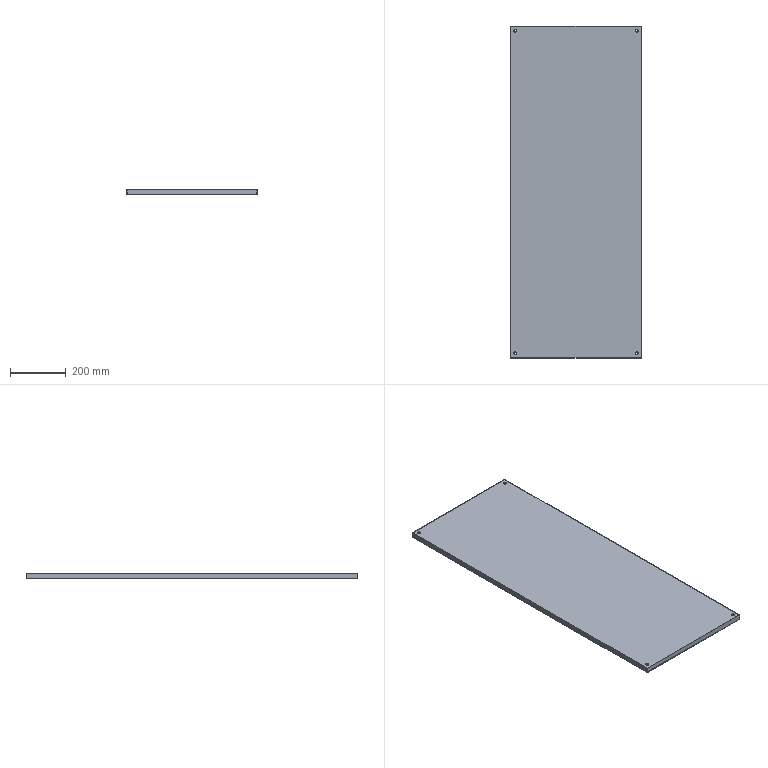Part | SolidWorks | features Extrusion 1, HoleWzd 1, ICE 1, Shell 1 | 1 solid | 32 faces | box 471 x 1196 x 20 mm | volume 1361647 mm3 | cylinder 16 | plane 16 | commonest cylinder face diameters 6.6 x8 11 x8
STEP:
#1=CARTESIAN_POINT('',(-213.,580.75,18.));
#2=VERTEX_POINT('',#1);
#3=CARTESIAN_POINT('',(-224.,580.75,18.));
#4=VERTEX_POINT('',#3);
#5=CARTESIAN_POINT('',(-218.5,580.75,18.));
#6=DIRECTION('',(0.,0.,-1.));
#7=DIRECTION('',(-1.,0.,0.));
#8=AXIS2_PLACEMENT_3D('',#5,#6,#7);
#9=CIRCLE('',#8,5.5);
#10=EDGE_CURVE('',#2,#4,#9,.T.);
#11=ORIENTED_EDGE('',*,*,#10,.T.);
#12=CARTESIAN_POINT('',(-224.,580.75,20.));
#13=VERTEX_POINT('',#12);
#14=CARTESIAN_POINT('',(-224.,580.75,20.));
#15=DIRECTION('',(0.,0.,1.));
#16=VECTOR('',#15,1000.);
#17=LINE('',#14,#16);
#18=EDGE_CURVE('',#4,#13,#17,.T.);
#19=ORIENTED_EDGE('',*,*,#18,.T.);
#20=CARTESIAN_POINT('',(-213.,580.75,20.));
#21=VERTEX_POINT('',#20);
#22=CARTESIAN_POINT('',(-218.5,580.75,20.));
#23=DIRECTION('',(0.,0.,1.));
#24=DIRECTION('',(1.,0.,0.));
#25=AXIS2_PLACEMENT_3D('',#22,#23,#24);
#26=CIRCLE('',#25,5.5);
#27=EDGE_CURVE('',#13,#21,#26,.T.);
#28=ORIENTED_EDGE('',*,*,#27,.T.);
#29=CARTESIAN_POINT('',(-213.,580.75,20.));
#30=DIRECTION('',(0.,0.,1.));
#31=VECTOR('',#30,1000.);
#32=LINE('',#29,#31);
#33=EDGE_CURVE('',#2,#21,#32,.T.);
#34=ORIENTED_EDGE('',*,*,#33,.F.);
#35=EDGE_LOOP('',(#11,#19,#28,#34));
#36=FACE_OUTER_BOUND('',#35,.T.);
#37=CARTESIAN_POINT('',(-218.5,580.75,20.));
#38=DIRECTION('',(0.,0.,1.));
#39=DIRECTION('',(1.,0.,0.));
#40=AXIS2_PLACEMENT_3D('',#37,#38,#39);
#41=CYLINDRICAL_SURFACE('',#40,5.5);
#42=ADVANCED_FACE('',(#36),#41,.F.);
#43=CARTESIAN_POINT('',(-221.8,580.75,0.));
#44=VERTEX_POINT('',#43);
#45=CARTESIAN_POINT('',(-215.2,580.75,0.));
#46=VERTEX_POINT('',#45);
#47=CARTESIAN_POINT('',(-218.5,580.75,0.));
#48=DIRECTION('',(0.,0.,1.));
#49=DIRECTION('',(1.,0.,0.));
#50=AXIS2_PLACEMENT_3D('',#47,#48,#49);
#51=CIRCLE('',#50,3.3);
#52=EDGE_CURVE('',#44,#46,#51,.T.);
#53=ORIENTED_EDGE('',*,*,#52,.F.);
#54=CARTESIAN_POINT('',(-221.8,580.75,2.));
#55=VERTEX_POINT('',#54);
#56=CARTESIAN_POINT('',(-221.8,580.75,20.));
#57=DIRECTION('',(0.,0.,1.));
#58=VECTOR('',#57,1000.);
#59=LINE('',#56,#58);
#60=EDGE_CURVE('',#44,#55,#59,.T.);
#61=ORIENTED_EDGE('',*,*,#60,.T.);
#62=CARTESIAN_POINT('',(-215.2,580.75,2.));
#63=VERTEX_POINT('',#62);
#64=CARTESIAN_POINT('',(-218.5,580.75,2.));
#65=DIRECTION('',(0.,0.,-1.));
#66=DIRECTION('',(-1.,0.,0.));
#67=AXIS2_PLACEMENT_3D('',#64,#65,#66);
#68=CIRCLE('',#67,3.3);
#69=EDGE_CURVE('',#63,#55,#68,.T.);
#70=ORIENTED_EDGE('',*,*,#69,.F.);
#71=CARTESIAN_POINT('',(-215.2,580.75,20.));
#72=DIRECTION('',(0.,0.,1.));
#73=VECTOR('',#72,1000.);
#74=LINE('',#71,#73);
#75=EDGE_CURVE('',#46,#63,#74,.T.);
#76=ORIENTED_EDGE('',*,*,#75,.F.);
#77=EDGE_LOOP('',(#53,#61,#70,#76));
#78=FACE_OUTER_BOUND('',#77,.T.);
#79=CARTESIAN_POINT('',(-218.5,580.75,20.));
#80=DIRECTION('',(0.,0.,1.));
#81=DIRECTION('',(1.,0.,0.));
#82=AXIS2_PLACEMENT_3D('',#79,#80,#81);
#83=CYLINDRICAL_SURFACE('',#82,3.3);
#84=ADVANCED_FACE('',(#78),#83,.F.);
#85=CARTESIAN_POINT('',(-213.,-580.75,18.));
#86=VERTEX_POINT('',#85);
#87=CARTESIAN_POINT('',(-224.,-580.75,18.));
#88=VERTEX_POINT('',#87);
#89=CARTESIAN_POINT('',(-218.5,-580.75,18.));
#90=DIRECTION('',(0.,0.,-1.));
#91=DIRECTION('',(-1.,0.,0.));
#92=AXIS2_PLACEMENT_3D('',#89,#90,#91);
#93=CIRCLE('',#92,5.5);
#94=EDGE_CURVE('',#86,#88,#93,.T.);
#95=ORIENTED_EDGE('',*,*,#94,.T.);
#96=CARTESIAN_POINT('',(-224.,-580.75,20.));
#97=VERTEX_POINT('',#96);
#98=CARTESIAN_POINT('',(-224.,-580.75,20.));
#99=DIRECTION('',(0.,0.,1.));
#100=VECTOR('',#99,1000.);
#101=LINE('',#98,#100);
#102=EDGE_CURVE('',#88,#97,#101,.T.);
#103=ORIENTED_EDGE('',*,*,#102,.T.);
#104=CARTESIAN_POINT('',(-213.,-580.75,20.));
#105=VERTEX_POINT('',#104);
#106=CARTESIAN_POINT('',(-218.5,-580.75,20.));
#107=DIRECTION('',(0.,0.,1.));
#108=DIRECTION('',(1.,0.,0.));
#109=AXIS2_PLACEMENT_3D('',#106,#107,#108);
#110=CIRCLE('',#109,5.5);
#111=EDGE_CURVE('',#97,#105,#110,.T.);
#112=ORIENTED_EDGE('',*,*,#111,.T.);
#113=CARTESIAN_POINT('',(-213.,-580.75,20.));
#114=DIRECTION('',(0.,0.,1.));
#115=VECTOR('',#114,1000.);
#116=LINE('',#113,#115);
#117=EDGE_CURVE('',#86,#105,#116,.T.);
#118=ORIENTED_EDGE('',*,*,#117,.F.);
#119=EDGE_LOOP('',(#95,#103,#112,#118));
#120=FACE_OUTER_BOUND('',#119,.T.);
#121=CARTESIAN_POINT('',(-218.5,-580.75,20.));
#122=DIRECTION('',(0.,0.,1.));
#123=DIRECTION('',(1.,0.,0.));
#124=AXIS2_PLACEMENT_3D('',#121,#122,#123);
#125=CYLINDRICAL_SURFACE('',#124,5.5);
#126=ADVANCED_FACE('',(#120),#125,.F.);
#127=CARTESIAN_POINT('',(-221.8,-580.75,0.));
#128=VERTEX_POINT('',#127);
#129=CARTESIAN_POINT('',(-215.2,-580.75,0.));
#130=VERTEX_POINT('',#129);
#131=CARTESIAN_POINT('',(-218.5,-580.75,0.));
#132=DIRECTION('',(0.,0.,1.));
#133=DIRECTION('',(1.,0.,0.));
#134=AXIS2_PLACEMENT_3D('',#131,#132,#133);
#135=CIRCLE('',#134,3.3);
#136=EDGE_CURVE('',#128,#130,#135,.T.);
#137=ORIENTED_EDGE('',*,*,#136,.F.);
#138=CARTESIAN_POINT('',(-221.8,-580.75,2.));
#139=VERTEX_POINT('',#138);
#140=CARTESIAN_POINT('',(-221.8,-580.75,20.));
#141=DIRECTION('',(0.,0.,1.));
#142=VECTOR('',#141,1000.);
#143=LINE('',#140,#142);
#144=EDGE_CURVE('',#128,#139,#143,.T.);
#145=ORIENTED_EDGE('',*,*,#144,.T.);
#146=CARTESIAN_POINT('',(-215.2,-580.75,2.));
#147=VERTEX_POINT('',#146);
#148=CARTESIAN_POINT('',(-218.5,-580.75,2.));
#149=DIRECTION('',(0.,0.,-1.));
#150=DIRECTION('',(-1.,0.,0.));
#151=AXIS2_PLACEMENT_3D('',#148,#149,#150);
#152=CIRCLE('',#151,3.3);
#153=EDGE_CURVE('',#147,#139,#152,.T.);
#154=ORIENTED_EDGE('',*,*,#153,.F.);
#155=CARTESIAN_POINT('',(-215.2,-580.75,20.));
#156=DIRECTION('',(0.,0.,1.));
#157=VECTOR('',#156,1000.);
#158=LINE('',#155,#157);
#159=EDGE_CURVE('',#130,#147,#158,.T.);
#160=ORIENTED_EDGE('',*,*,#159,.F.);
#161=EDGE_LOOP('',(#137,#145,#154,#160));
#162=FACE_OUTER_BOUND('',#161,.T.);
#163=CARTESIAN_POINT('',(-218.5,-580.75,20.));
#164=DIRECTION('',(0.,0.,1.));
#165=DIRECTION('',(1.,0.,0.));
#166=AXIS2_PLACEMENT_3D('',#163,#164,#165);
#167=CYLINDRICAL_SURFACE('',#166,3.3);
#168=ADVANCED_FACE('',(#162),#167,.F.);
#169=CARTESIAN_POINT('',(215.2,-580.75,0.));
#170=VERTEX_POINT('',#169);
#171=CARTESIAN_POINT('',(221.8,-580.75,0.));
#172=VERTEX_POINT('',#171);
#173=CARTESIAN_POINT('',(218.5,-580.75,0.));
#174=DIRECTION('',(0.,0.,1.));
#175=DIRECTION('',(1.,0.,0.));
#176=AXIS2_PLACEMENT_3D('',#173,#174,#175);
#177=CIRCLE('',#176,3.3);
#178=EDGE_CURVE('',#170,#172,#177,.T.);
#179=ORIENTED_EDGE('',*,*,#178,.F.);
#180=CARTESIAN_POINT('',(215.2,-580.75,2.));
#181=VERTEX_POINT('',#180);
#182=CARTESIAN_POINT('',(215.2,-580.75,20.));
#183=DIRECTION('',(0.,0.,1.));
#184=VECTOR('',#183,1000.);
#185=LINE('',#182,#184);
#186=EDGE_CURVE('',#170,#181,#185,.T.);
#187=ORIENTED_EDGE('',*,*,#186,.T.);
#188=CARTESIAN_POINT('',(221.8,-580.75,2.));
#189=VERTEX_POINT('',#188);
#190=CARTESIAN_POINT('',(218.5,-580.75,2.));
#191=DIRECTION('',(0.,0.,-1.));
#192=DIRECTION('',(-1.,0.,0.));
#193=AXIS2_PLACEMENT_3D('',#190,#191,#192);
#194=CIRCLE('',#193,3.3);
#195=EDGE_CURVE('',#189,#181,#194,.T.);
#196=ORIENTED_EDGE('',*,*,#195,.F.);
#197=CARTESIAN_POINT('',(221.8,-580.75,20.));
#198=DIRECTION('',(0.,0.,1.));
#199=VECTOR('',#198,1000.);
#200=LINE('',#197,#199);
#201=EDGE_CURVE('',#172,#189,#200,.T.);
#202=ORIENTED_EDGE('',*,*,#201,.F.);
#203=EDGE_LOOP('',(#179,#187,#196,#202));
#204=FACE_OUTER_BOUND('',#203,.T.);
#205=CARTESIAN_POINT('',(218.5,-580.75,20.));
#206=DIRECTION('',(0.,0.,1.));
#207=DIRECTION('',(1.,0.,0.));
#208=AXIS2_PLACEMENT_3D('',#205,#206,#207);
#209=CYLINDRICAL_SURFACE('',#208,3.3);
#210=ADVANCED_FACE('',(#204),#209,.F.);
#211=CARTESIAN_POINT('',(224.,-580.75,18.));
#212=VERTEX_POINT('',#211);
#213=CARTESIAN_POINT('',(213.,-580.75,18.));
#214=VERTEX_POINT('',#213);
#215=CARTESIAN_POINT('',(218.5,-580.75,18.));
#216=DIRECTION('',(0.,0.,-1.));
#217=DIRECTION('',(-1.,0.,0.));
#218=AXIS2_PLACEMENT_3D('',#215,#216,#217);
#219=CIRCLE('',#218,5.5);
#220=EDGE_CURVE('',#212,#214,#219,.T.);
#221=ORIENTED_EDGE('',*,*,#220,.T.);
#222=CARTESIAN_POINT('',(213.,-580.75,20.));
#223=VERTEX_POINT('',#222);
#224=CARTESIAN_POINT('',(213.,-580.75,20.));
#225=DIRECTION('',(0.,0.,1.));
#226=VECTOR('',#225,1000.);
#227=LINE('',#224,#226);
#228=EDGE_CURVE('',#214,#223,#227,.T.);
#229=ORIENTED_EDGE('',*,*,#228,.T.);
#230=CARTESIAN_POINT('',(224.,-580.75,20.));
#231=VERTEX_POINT('',#230);
#232=CARTESIAN_POINT('',(218.5,-580.75,20.));
#233=DIRECTION('',(0.,0.,1.));
#234=DIRECTION('',(1.,0.,0.));
#235=AXIS2_PLACEMENT_3D('',#232,#233,#234);
#236=CIRCLE('',#235,5.5);
#237=EDGE_CURVE('',#223,#231,#236,.T.);
#238=ORIENTED_EDGE('',*,*,#237,.T.);
#239=CARTESIAN_POINT('',(224.,-580.75,20.));
#240=DIRECTION('',(0.,0.,1.));
#241=VECTOR('',#240,1000.);
#242=LINE('',#239,#241);
#243=EDGE_CURVE('',#212,#231,#242,.T.);
#244=ORIENTED_EDGE('',*,*,#243,.F.);
#245=EDGE_LOOP('',(#221,#229,#238,#244));
#246=FACE_OUTER_BOUND('',#245,.T.);
#247=CARTESIAN_POINT('',(218.5,-580.75,20.));
#248=DIRECTION('',(0.,0.,1.));
#249=DIRECTION('',(1.,0.,0.));
#250=AXIS2_PLACEMENT_3D('',#247,#248,#249);
#251=CYLINDRICAL_SURFACE('',#250,5.5);
#252=ADVANCED_FACE('',(#246),#251,.F.);
#253=CARTESIAN_POINT('',(224.,580.75,18.));
#254=VERTEX_POINT('',#253);
#255=CARTESIAN_POINT('',(213.,580.75,18.));
#256=VERTEX_POINT('',#255);
#257=CARTESIAN_POINT('',(218.5,580.75,18.));
#258=DIRECTION('',(0.,0.,-1.));
#259=DIRECTION('',(-1.,0.,0.));
#260=AXIS2_PLACEMENT_3D('',#257,#258,#259);
#261=CIRCLE('',#260,5.5);
#262=EDGE_CURVE('',#254,#256,#261,.T.);
#263=ORIENTED_EDGE('',*,*,#262,.T.);
#264=CARTESIAN_POINT('',(213.,580.75,20.));
#265=VERTEX_POINT('',#264);
#266=CARTESIAN_POINT('',(213.,580.75,20.));
#267=DIRECTION('',(0.,0.,1.));
#268=VECTOR('',#267,1000.);
#269=LINE('',#266,#268);
#270=EDGE_CURVE('',#256,#265,#269,.T.);
#271=ORIENTED_EDGE('',*,*,#270,.T.);
#272=CARTESIAN_POINT('',(224.,580.75,20.));
#273=VERTEX_POINT('',#272);
#274=CARTESIAN_POINT('',(218.5,580.75,20.));
#275=DIRECTION('',(0.,0.,1.));
#276=DIRECTION('',(1.,0.,0.));
#277=AXIS2_PLACEMENT_3D('',#274,#275,#276);
#278=CIRCLE('',#277,5.5);
#279=EDGE_CURVE('',#265,#273,#278,.T.);
#280=ORIENTED_EDGE('',*,*,#279,.T.);
#281=CARTESIAN_POINT('',(224.,580.75,20.));
#282=DIRECTION('',(0.,0.,1.));
#283=VECTOR('',#282,1000.);
#284=LINE('',#281,#283);
#285=EDGE_CURVE('',#254,#273,#284,.T.);
#286=ORIENTED_EDGE('',*,*,#285,.F.);
#287=EDGE_LOOP('',(#263,#271,#280,#286));
#288=FACE_OUTER_BOUND('',#287,.T.);
#289=CARTESIAN_POINT('',(218.5,580.75,20.));
#290=DIRECTION('',(0.,0.,1.));
#291=DIRECTION('',(1.,0.,0.));
#292=AXIS2_PLACEMENT_3D('',#289,#290,#291);
#293=CYLINDRICAL_SURFACE('',#292,5.5);
#294=ADVANCED_FACE('',(#288),#293,.F.);
#295=CARTESIAN_POINT('',(215.2,580.75,0.));
#296=VERTEX_POINT('',#295);
#297=CARTESIAN_POINT('',(221.8,580.75,0.));
#298=VERTEX_POINT('',#297);
#299=CARTESIAN_POINT('',(218.5,580.75,0.));
#300=DIRECTION('',(0.,0.,1.));
#301=DIRECTION('',(1.,0.,0.));
#302=AXIS2_PLACEMENT_3D('',#299,#300,#301);
#303=CIRCLE('',#302,3.3);
#304=EDGE_CURVE('',#296,#298,#303,.T.);
#305=ORIENTED_EDGE('',*,*,#304,.F.);
#306=CARTESIAN_POINT('',(215.2,580.75,2.));
#307=VERTEX_POINT('',#306);
#308=CARTESIAN_POINT('',(215.2,580.75,20.));
#309=DIRECTION('',(0.,0.,1.));
#310=VECTOR('',#309,1000.);
#311=LINE('',#308,#310);
#312=EDGE_CURVE('',#296,#307,#311,.T.);
#313=ORIENTED_EDGE('',*,*,#312,.T.);
#314=CARTESIAN_POINT('',(221.8,580.75,2.));
#315=VERTEX_POINT('',#314);
#316=CARTESIAN_POINT('',(218.5,580.75,2.));
#317=DIRECTION('',(0.,0.,-1.));
#318=DIRECTION('',(-1.,0.,0.));
#319=AXIS2_PLACEMENT_3D('',#316,#317,#318);
#320=CIRCLE('',#319,3.3);
#321=EDGE_CURVE('',#315,#307,#320,.T.);
#322=ORIENTED_EDGE('',*,*,#321,.F.);
#323=CARTESIAN_POINT('',(221.8,580.75,20.));
#324=DIRECTION('',(0.,0.,1.));
#325=VECTOR('',#324,1000.);
#326=LINE('',#323,#325);
#327=EDGE_CURVE('',#298,#315,#326,.T.);
#328=ORIENTED_EDGE('',*,*,#327,.F.);
#329=EDGE_LOOP('',(#305,#313,#322,#328));
#330=FACE_OUTER_BOUND('',#329,.T.);
#331=CARTESIAN_POINT('',(218.5,580.75,20.));
#332=DIRECTION('',(0.,0.,1.));
#333=DIRECTION('',(1.,0.,0.));
#334=AXIS2_PLACEMENT_3D('',#331,#332,#333);
#335=CYLINDRICAL_SURFACE('',#334,3.3);
#336=ADVANCED_FACE('',(#330),#335,.F.);
#337=CARTESIAN_POINT('',(-218.5,580.75,0.));
#338=DIRECTION('',(0.,0.,1.));
#339=DIRECTION('',(1.,0.,0.));
#340=AXIS2_PLACEMENT_3D('',#337,#338,#339);
#341=CIRCLE('',#340,3.3);
#342=EDGE_CURVE('',#46,#44,#341,.T.);
#343=ORIENTED_EDGE('',*,*,#342,.T.);
#344=ORIENTED_EDGE('',*,*,#52,.T.);
#345=EDGE_LOOP('',(#343,#344));
#346=FACE_BOUND('',#345,.T.);
#347=CARTESIAN_POINT('',(-218.5,-580.75,0.));
#348=DIRECTION('',(0.,0.,1.));
#349=DIRECTION('',(1.,0.,0.));
#350=AXIS2_PLACEMENT_3D('',#347,#348,#349);
#351=CIRCLE('',#350,3.3);
#352=EDGE_CURVE('',#130,#128,#351,.T.);
#353=ORIENTED_EDGE('',*,*,#352,.T.);
#354=ORIENTED_EDGE('',*,*,#136,.T.);
#355=EDGE_LOOP('',(#353,#354));
#356=FACE_BOUND('',#355,.T.);
#357=CARTESIAN_POINT('',(218.5,-580.75,0.));
#358=DIRECTION('',(0.,0.,1.));
#359=DIRECTION('',(1.,0.,0.));
#360=AXIS2_PLACEMENT_3D('',#357,#358,#359);
#361=CIRCLE('',#360,3.3);
#362=EDGE_CURVE('',#172,#170,#361,.T.);
#363=ORIENTED_EDGE('',*,*,#362,.T.);
#364=ORIENTED_EDGE('',*,*,#178,.T.);
#365=EDGE_LOOP('',(#363,#364));
#366=FACE_BOUND('',#365,.T.);
#367=CARTESIAN_POINT('',(215.5,-577.75,0.));
#368=VERTEX_POINT('',#367);
#369=CARTESIAN_POINT('',(-215.5,-577.75,0.));
#370=VERTEX_POINT('',#369);
#371=CARTESIAN_POINT('',(215.5,-577.75,0.));
#372=DIRECTION('',(-1.,0.,0.));
#373=VECTOR('',#372,1000.);
#374=LINE('',#371,#373);
#375=EDGE_CURVE('',#368,#370,#374,.T.);
#376=ORIENTED_EDGE('',*,*,#375,.F.);
#377=CARTESIAN_POINT('',(215.5,577.75,0.));
#378=VERTEX_POINT('',#377);
#379=CARTESIAN_POINT('',(215.5,-577.75,0.));
#380=DIRECTION('',(0.,1.,0.));
#381=VECTOR('',#380,1000.);
#382=LINE('',#379,#381);
#383=EDGE_CURVE('',#368,#378,#382,.T.);
#384=ORIENTED_EDGE('',*,*,#383,.T.);
#385=CARTESIAN_POINT('',(-215.5,577.75,0.));
#386=VERTEX_POINT('',#385);
#387=CARTESIAN_POINT('',(215.5,577.75,0.));
#388=DIRECTION('',(-1.,0.,0.));
#389=VECTOR('',#388,1000.);
#390=LINE('',#387,#389);
#391=EDGE_CURVE('',#378,#386,#390,.T.);
#392=ORIENTED_EDGE('',*,*,#391,.T.);
#393=CARTESIAN_POINT('',(-215.5,-577.75,0.));
#394=DIRECTION('',(0.,1.,0.));
#395=VECTOR('',#394,1000.);
#396=LINE('',#393,#395);
#397=EDGE_CURVE('',#370,#386,#396,.T.);
#398=ORIENTED_EDGE('',*,*,#397,.F.);
#399=EDGE_LOOP('',(#376,#384,#392,#398));
#400=FACE_BOUND('',#399,.T.);
#401=CARTESIAN_POINT('',(235.5,-597.75,0.));
#402=VERTEX_POINT('',#401);
#403=CARTESIAN_POINT('',(235.5,597.75,0.));
#404=VERTEX_POINT('',#403);
#405=CARTESIAN_POINT('',(235.5,-597.75,0.));
#406=DIRECTION('',(0.,1.,0.));
#407=VECTOR('',#406,1000.);
#408=LINE('',#405,#407);
#409=EDGE_CURVE('',#402,#404,#408,.T.);
#410=ORIENTED_EDGE('',*,*,#409,.F.);
#411=CARTESIAN_POINT('',(-235.5,-597.75,0.));
#412=VERTEX_POINT('',#411);
#413=CARTESIAN_POINT('',(-235.5,-597.75,0.));
#414=DIRECTION('',(1.,0.,0.));
#415=VECTOR('',#414,1000.);
#416=LINE('',#413,#415);
#417=EDGE_CURVE('',#412,#402,#416,.T.);
#418=ORIENTED_EDGE('',*,*,#417,.F.);
#419=CARTESIAN_POINT('',(-235.5,597.75,0.));
#420=VERTEX_POINT('',#419);
#421=CARTESIAN_POINT('',(-235.5,-597.75,0.));
#422=DIRECTION('',(0.,-1.,0.));
#423=VECTOR('',#422,1000.);
#424=LINE('',#421,#423);
#425=EDGE_CURVE('',#420,#412,#424,.T.);
#426=ORIENTED_EDGE('',*,*,#425,.F.);
#427=CARTESIAN_POINT('',(-235.5,597.75,0.));
#428=DIRECTION('',(-1.,0.,0.));
#429=VECTOR('',#428,1000.);
#430=LINE('',#427,#429);
#431=EDGE_CURVE('',#404,#420,#430,.T.);
#432=ORIENTED_EDGE('',*,*,#431,.F.);
#433=EDGE_LOOP('',(#410,#418,#426,#432));
#434=FACE_OUTER_BOUND('',#433,.T.);
#435=CARTESIAN_POINT('',(218.5,580.75,0.));
#436=DIRECTION('',(0.,0.,1.));
#437=DIRECTION('',(1.,0.,0.));
#438=AXIS2_PLACEMENT_3D('',#435,#436,#437);
#439=CIRCLE('',#438,3.3);
#440=EDGE_CURVE('',#298,#296,#439,.T.);
#441=ORIENTED_EDGE('',*,*,#440,.T.);
#442=ORIENTED_EDGE('',*,*,#304,.T.);
#443=EDGE_LOOP('',(#441,#442));
#444=FACE_BOUND('',#443,.T.);
#445=CARTESIAN_POINT('',(0.,0.,0.));
#446=DIRECTION('',(0.,0.,-1.));
#447=DIRECTION('',(-1.,0.,0.));
#448=AXIS2_PLACEMENT_3D('',#445,#446,#447);
#449=PLANE('',#448);
#450=ADVANCED_FACE('',(#346,#356,#366,#400,#434,#444),#449,.T.);
#451=ORIENTED_EDGE('',*,*,#409,.T.);
#452=CARTESIAN_POINT('',(235.5,597.75,20.));
#453=VERTEX_POINT('',#452);
#454=CARTESIAN_POINT('',(235.5,597.75,20.));
#455=DIRECTION('',(0.,0.,-1.));
#456=VECTOR('',#455,1000.);
#457=LINE('',#454,#456);
#458=EDGE_CURVE('',#453,#404,#457,.T.);
#459=ORIENTED_EDGE('',*,*,#458,.F.);
#460=CARTESIAN_POINT('',(235.5,-597.75,20.));
#461=VERTEX_POINT('',#460);
#462=CARTESIAN_POINT('',(235.5,-597.75,20.));
#463=DIRECTION('',(0.,1.,0.));
#464=VECTOR('',#463,1000.);
#465=LINE('',#462,#464);
#466=EDGE_CURVE('',#461,#453,#465,.T.);
#467=ORIENTED_EDGE('',*,*,#466,.F.);
#468=CARTESIAN_POINT('',(235.5,-597.75,20.));
#469=DIRECTION('',(0.,0.,-1.));
#470=VECTOR('',#469,1000.);
#471=LINE('',#468,#470);
#472=EDGE_CURVE('',#461,#402,#471,.T.);
#473=ORIENTED_EDGE('',*,*,#472,.T.);
#474=EDGE_LOOP('',(#451,#459,#467,#473));
#475=FACE_OUTER_BOUND('',#474,.T.);
#476=CARTESIAN_POINT('',(235.5,-597.75,20.));
#477=DIRECTION('',(-1.,0.,0.));
#478=DIRECTION('',(0.,0.,1.));
#479=AXIS2_PLACEMENT_3D('',#476,#477,#478);
#480=PLANE('',#479);
#481=ADVANCED_FACE('',(#475),#480,.F.);
#482=ORIENTED_EDGE('',*,*,#431,.T.);
#483=CARTESIAN_POINT('',(-235.5,597.75,20.));
#484=VERTEX_POINT('',#483);
#485=CARTESIAN_POINT('',(-235.5,597.75,20.));
#486=DIRECTION('',(0.,0.,-1.));
#487=VECTOR('',#486,1000.);
#488=LINE('',#485,#487);
#489=EDGE_CURVE('',#484,#420,#488,.T.);
#490=ORIENTED_EDGE('',*,*,#489,.F.);
#491=CARTESIAN_POINT('',(-235.5,597.75,20.));
#492=DIRECTION('',(-1.,0.,0.));
#493=VECTOR('',#492,1000.);
#494=LINE('',#491,#493);
#495=EDGE_CURVE('',#453,#484,#494,.T.);
#496=ORIENTED_EDGE('',*,*,#495,.F.);
#497=ORIENTED_EDGE('',*,*,#458,.T.);
#498=EDGE_LOOP('',(#482,#490,#496,#497));
#499=FACE_OUTER_BOUND('',#498,.T.);
#500=CARTESIAN_POINT('',(-235.5,597.75,20.));
#501=DIRECTION('',(0.,-1.,0.));
#502=DIRECTION('',(0.,0.,-1.));
#503=AXIS2_PLACEMENT_3D('',#500,#501,#502);
#504=PLANE('',#503);
#505=ADVANCED_FACE('',(#499),#504,.F.);
#506=ORIENTED_EDGE('',*,*,#425,.T.);
#507=CARTESIAN_POINT('',(-235.5,-597.75,20.));
#508=VERTEX_POINT('',#507);
#509=CARTESIAN_POINT('',(-235.5,-597.75,20.));
#510=DIRECTION('',(0.,0.,-1.));
#511=VECTOR('',#510,1000.);
#512=LINE('',#509,#511);
#513=EDGE_CURVE('',#508,#412,#512,.T.);
#514=ORIENTED_EDGE('',*,*,#513,.F.);
#515=CARTESIAN_POINT('',(-235.5,-597.75,20.));
#516=DIRECTION('',(0.,-1.,0.));
#517=VECTOR('',#516,1000.);
#518=LINE('',#515,#517);
#519=EDGE_CURVE('',#484,#508,#518,.T.);
#520=ORIENTED_EDGE('',*,*,#519,.F.);
#521=ORIENTED_EDGE('',*,*,#489,.T.);
#522=EDGE_LOOP('',(#506,#514,#520,#521));
#523=FACE_OUTER_BOUND('',#522,.T.);
#524=CARTESIAN_POINT('',(-235.5,-597.75,20.));
#525=DIRECTION('',(1.,0.,0.));
#526=DIRECTION('',(0.,0.,-1.));
#527=AXIS2_PLACEMENT_3D('',#524,#525,#526);
#528=PLANE('',#527);
#529=ADVANCED_FACE('',(#523),#528,.F.);
#530=ORIENTED_EDGE('',*,*,#417,.T.);
#531=ORIENTED_EDGE('',*,*,#472,.F.);
#532=CARTESIAN_POINT('',(-235.5,-597.75,20.));
#533=DIRECTION('',(1.,0.,0.));
#534=VECTOR('',#533,1000.);
#535=LINE('',#532,#534);
#536=EDGE_CURVE('',#508,#461,#535,.T.);
#537=ORIENTED_EDGE('',*,*,#536,.F.);
#538=ORIENTED_EDGE('',*,*,#513,.T.);
#539=EDGE_LOOP('',(#530,#531,#537,#538));
#540=FACE_OUTER_BOUND('',#539,.T.);
#541=CARTESIAN_POINT('',(-235.5,-597.75,20.));
#542=DIRECTION('',(0.,1.,0.));
#543=DIRECTION('',(0.,0.,1.));
#544=AXIS2_PLACEMENT_3D('',#541,#542,#543);
#545=PLANE('',#544);
#546=ADVANCED_FACE('',(#540),#545,.F.);
#547=CARTESIAN_POINT('',(-218.5,580.75,20.));
#548=DIRECTION('',(0.,0.,1.));
#549=DIRECTION('',(1.,0.,0.));
#550=AXIS2_PLACEMENT_3D('',#547,#548,#549);
#551=CIRCLE('',#550,5.5);
#552=EDGE_CURVE('',#21,#13,#551,.T.);
#553=ORIENTED_EDGE('',*,*,#552,.F.);
#554=ORIENTED_EDGE('',*,*,#27,.F.);
#555=EDGE_LOOP('',(#553,#554));
#556=FACE_BOUND('',#555,.T.);
#557=CARTESIAN_POINT('',(-218.5,-580.75,20.));
#558=DIRECTION('',(0.,0.,1.));
#559=DIRECTION('',(1.,0.,0.));
#560=AXIS2_PLACEMENT_3D('',#557,#558,#559);
#561=CIRCLE('',#560,5.5);
#562=EDGE_CURVE('',#105,#97,#561,.T.);
#563=ORIENTED_EDGE('',*,*,#562,.F.);
#564=ORIENTED_EDGE('',*,*,#111,.F.);
#565=EDGE_LOOP('',(#563,#564));
#566=FACE_BOUND('',#565,.T.);
#567=CARTESIAN_POINT('',(218.5,-580.75,20.));
#568=DIRECTION('',(0.,0.,1.));
#569=DIRECTION('',(1.,0.,0.));
#570=AXIS2_PLACEMENT_3D('',#567,#568,#569);
#571=CIRCLE('',#570,5.5);
#572=EDGE_CURVE('',#231,#223,#571,.T.);
#573=ORIENTED_EDGE('',*,*,#572,.F.);
#574=ORIENTED_EDGE('',*,*,#237,.F.);
#575=EDGE_LOOP('',(#573,#574));
#576=FACE_BOUND('',#575,.T.);
#577=CARTESIAN_POINT('',(218.5,580.75,20.));
#578=DIRECTION('',(0.,0.,1.));
#579=DIRECTION('',(1.,0.,0.));
#580=AXIS2_PLACEMENT_3D('',#577,#578,#579);
#581=CIRCLE('',#580,5.5);
#582=EDGE_CURVE('',#273,#265,#581,.T.);
#583=ORIENTED_EDGE('',*,*,#582,.F.);
#584=ORIENTED_EDGE('',*,*,#279,.F.);
#585=EDGE_LOOP('',(#583,#584));
#586=FACE_BOUND('',#585,.T.);
#587=ORIENTED_EDGE('',*,*,#466,.T.);
#588=ORIENTED_EDGE('',*,*,#495,.T.);
#589=ORIENTED_EDGE('',*,*,#519,.T.);
#590=ORIENTED_EDGE('',*,*,#536,.T.);
#591=EDGE_LOOP('',(#587,#588,#589,#590));
#592=FACE_OUTER_BOUND('',#591,.T.);
#593=CARTESIAN_POINT('',(0.,0.,20.));
#594=DIRECTION('',(0.,0.,-1.));
#595=DIRECTION('',(-1.,0.,0.));
#596=AXIS2_PLACEMENT_3D('',#593,#594,#595);
#597=PLANE('',#596);
#598=ADVANCED_FACE('',(#556,#566,#576,#586,#592),#597,.F.);
#599=ORIENTED_EDGE('',*,*,#383,.F.);
#600=CARTESIAN_POINT('',(215.5,-577.75,2.));
#601=VERTEX_POINT('',#600);
#602=CARTESIAN_POINT('',(215.5,-577.75,2.));
#603=DIRECTION('',(0.,0.,-1.));
#604=VECTOR('',#603,1000.);
#605=LINE('',#602,#604);
#606=EDGE_CURVE('',#601,#368,#605,.T.);
#607=ORIENTED_EDGE('',*,*,#606,.F.);
#608=CARTESIAN_POINT('',(215.5,577.75,2.));
#609=VERTEX_POINT('',#608);
#610=CARTESIAN_POINT('',(215.5,-577.75,2.));
#611=DIRECTION('',(0.,1.,0.));
#612=VECTOR('',#611,1000.);
#613=LINE('',#610,#612);
#614=EDGE_CURVE('',#601,#609,#613,.T.);
#615=ORIENTED_EDGE('',*,*,#614,.T.);
#616=CARTESIAN_POINT('',(215.5,577.75,2.));
#617=DIRECTION('',(0.,0.,-1.));
#618=VECTOR('',#617,1000.);
#619=LINE('',#616,#618);
#620=EDGE_CURVE('',#609,#378,#619,.T.);
#621=ORIENTED_EDGE('',*,*,#620,.T.);
#622=EDGE_LOOP('',(#599,#607,#615,#621));
#623=FACE_OUTER_BOUND('',#622,.T.);
#624=CARTESIAN_POINT('',(215.5,-577.75,2.));
#625=DIRECTION('',(-1.,0.,0.));
#626=DIRECTION('',(0.,0.,1.));
#627=AXIS2_PLACEMENT_3D('',#624,#625,#626);
#628=PLANE('',#627);
#629=ADVANCED_FACE('',(#623),#628,.T.);
#630=ORIENTED_EDGE('',*,*,#391,.F.);
#631=ORIENTED_EDGE('',*,*,#620,.F.);
#632=CARTESIAN_POINT('',(-215.5,577.75,2.));
#633=VERTEX_POINT('',#632);
#634=CARTESIAN_POINT('',(215.5,577.75,2.));
#635=DIRECTION('',(-1.,0.,0.));
#636=VECTOR('',#635,1000.);
#637=LINE('',#634,#636);
#638=EDGE_CURVE('',#609,#633,#637,.T.);
#639=ORIENTED_EDGE('',*,*,#638,.T.);
#640=CARTESIAN_POINT('',(-215.5,577.75,2.));
#641=DIRECTION('',(0.,0.,-1.));
#642=VECTOR('',#641,1000.);
#643=LINE('',#640,#642);
#644=EDGE_CURVE('',#633,#386,#643,.T.);
#645=ORIENTED_EDGE('',*,*,#644,.T.);
#646=EDGE_LOOP('',(#630,#631,#639,#645));
#647=FACE_OUTER_BOUND('',#646,.T.);
#648=CARTESIAN_POINT('',(215.5,577.75,2.));
#649=DIRECTION('',(0.,-1.,0.));
#650=DIRECTION('',(0.,0.,-1.));
#651=AXIS2_PLACEMENT_3D('',#648,#649,#650);
#652=PLANE('',#651);
#653=ADVANCED_FACE('',(#647),#652,.T.);
#654=ORIENTED_EDGE('',*,*,#397,.T.);
#655=ORIENTED_EDGE('',*,*,#644,.F.);
#656=CARTESIAN_POINT('',(-215.5,-577.75,2.));
#657=VERTEX_POINT('',#656);
#658=CARTESIAN_POINT('',(-215.5,-577.75,2.));
#659=DIRECTION('',(0.,1.,0.));
#660=VECTOR('',#659,1000.);
#661=LINE('',#658,#660);
#662=EDGE_CURVE('',#657,#633,#661,.T.);
#663=ORIENTED_EDGE('',*,*,#662,.F.);
#664=CARTESIAN_POINT('',(-215.5,-577.75,2.));
#665=DIRECTION('',(0.,0.,-1.));
#666=VECTOR('',#665,1000.);
#667=LINE('',#664,#666);
#668=EDGE_CURVE('',#657,#370,#667,.T.);
#669=ORIENTED_EDGE('',*,*,#668,.T.);
#670=EDGE_LOOP('',(#654,#655,#663,#669));
#671=FACE_OUTER_BOUND('',#670,.T.);
#672=CARTESIAN_POINT('',(-215.5,-577.75,2.));
#673=DIRECTION('',(-1.,0.,0.));
#674=DIRECTION('',(0.,0.,1.));
#675=AXIS2_PLACEMENT_3D('',#672,#673,#674);
#676=PLANE('',#675);
#677=ADVANCED_FACE('',(#671),#676,.F.);
#678=ORIENTED_EDGE('',*,*,#375,.T.);
#679=ORIENTED_EDGE('',*,*,#668,.F.);
#680=CARTESIAN_POINT('',(215.5,-577.75,2.));
#681=DIRECTION('',(-1.,0.,0.));
#682=VECTOR('',#681,1000.);
#683=LINE('',#680,#682);
#684=EDGE_CURVE('',#601,#657,#683,.T.);
#685=ORIENTED_EDGE('',*,*,#684,.F.);
#686=ORIENTED_EDGE('',*,*,#606,.T.);
#687=EDGE_LOOP('',(#678,#679,#685,#686));
#688=FACE_OUTER_BOUND('',#687,.T.);
#689=CARTESIAN_POINT('',(215.5,-577.75,2.));
#690=DIRECTION('',(0.,-1.,0.));
#691=DIRECTION('',(0.,0.,-1.));
#692=AXIS2_PLACEMENT_3D('',#689,#690,#691);
#693=PLANE('',#692);
#694=ADVANCED_FACE('',(#688),#693,.F.);
#695=ORIENTED_EDGE('',*,*,#69,.T.);
#696=CARTESIAN_POINT('',(-218.5,580.75,2.));
#697=DIRECTION('',(0.,0.,-1.));
#698=DIRECTION('',(-1.,0.,0.));
#699=AXIS2_PLACEMENT_3D('',#696,#697,#698);
#700=CIRCLE('',#699,3.3);
#701=EDGE_CURVE('',#55,#63,#700,.T.);
#702=ORIENTED_EDGE('',*,*,#701,.T.);
#703=EDGE_LOOP('',(#695,#702));
#704=FACE_BOUND('',#703,.T.);
#705=ORIENTED_EDGE('',*,*,#153,.T.);
#706=CARTESIAN_POINT('',(-218.5,-580.75,2.));
#707=DIRECTION('',(0.,0.,-1.));
#708=DIRECTION('',(-1.,0.,0.));
#709=AXIS2_PLACEMENT_3D('',#706,#707,#708);
#710=CIRCLE('',#709,3.3);
#711=EDGE_CURVE('',#139,#147,#710,.T.);
#712=ORIENTED_EDGE('',*,*,#711,.T.);
#713=EDGE_LOOP('',(#705,#712));
#714=FACE_BOUND('',#713,.T.);
#715=ORIENTED_EDGE('',*,*,#195,.T.);
#716=CARTESIAN_POINT('',(218.5,-580.75,2.));
#717=DIRECTION('',(0.,0.,-1.));
#718=DIRECTION('',(-1.,0.,0.));
#719=AXIS2_PLACEMENT_3D('',#716,#717,#718);
#720=CIRCLE('',#719,3.3);
#721=EDGE_CURVE('',#181,#189,#720,.T.);
#722=ORIENTED_EDGE('',*,*,#721,.T.);
#723=EDGE_LOOP('',(#715,#722));
#724=FACE_BOUND('',#723,.T.);
#725=ORIENTED_EDGE('',*,*,#321,.T.);
#726=CARTESIAN_POINT('',(218.5,580.75,2.));
#727=DIRECTION('',(0.,0.,-1.));
#728=DIRECTION('',(-1.,0.,0.));
#729=AXIS2_PLACEMENT_3D('',#726,#727,#728);
#730=CIRCLE('',#729,3.3);
#731=EDGE_CURVE('',#307,#315,#730,.T.);
#732=ORIENTED_EDGE('',*,*,#731,.T.);
#733=EDGE_LOOP('',(#725,#732));
#734=FACE_BOUND('',#733,.T.);
#735=CARTESIAN_POINT('',(233.5,-595.75,2.));
#736=VERTEX_POINT('',#735);
#737=CARTESIAN_POINT('',(233.5,595.75,2.));
#738=VERTEX_POINT('',#737);
#739=CARTESIAN_POINT('',(233.5,0.,2.));
#740=DIRECTION('',(0.,1.,0.));
#741=VECTOR('',#740,1000.);
#742=LINE('',#739,#741);
#743=EDGE_CURVE('',#736,#738,#742,.T.);
#744=ORIENTED_EDGE('',*,*,#743,.T.);
#745=CARTESIAN_POINT('',(-233.5,595.75,2.));
#746=VERTEX_POINT('',#745);
#747=CARTESIAN_POINT('',(0.,595.75,2.));
#748=DIRECTION('',(-1.,0.,0.));
#749=VECTOR('',#748,1000.);
#750=LINE('',#747,#749);
#751=EDGE_CURVE('',#738,#746,#750,.T.);
#752=ORIENTED_EDGE('',*,*,#751,.T.);
#753=CARTESIAN_POINT('',(-233.5,-595.75,2.));
#754=VERTEX_POINT('',#753);
#755=CARTESIAN_POINT('',(-233.5,0.,2.));
#756=DIRECTION('',(0.,-1.,0.));
#757=VECTOR('',#756,1000.);
#758=LINE('',#755,#757);
#759=EDGE_CURVE('',#746,#754,#758,.T.);
#760=ORIENTED_EDGE('',*,*,#759,.T.);
#761=CARTESIAN_POINT('',(0.,-595.75,2.));
#762=DIRECTION('',(1.,0.,0.));
#763=VECTOR('',#762,1000.);
#764=LINE('',#761,#763);
#765=EDGE_CURVE('',#754,#736,#764,.T.);
#766=ORIENTED_EDGE('',*,*,#765,.T.);
#767=EDGE_LOOP('',(#744,#752,#760,#766));
#768=FACE_OUTER_BOUND('',#767,.T.);
#769=ORIENTED_EDGE('',*,*,#684,.T.);
#770=ORIENTED_EDGE('',*,*,#662,.T.);
#771=ORIENTED_EDGE('',*,*,#638,.F.);
#772=ORIENTED_EDGE('',*,*,#614,.F.);
#773=EDGE_LOOP('',(#769,#770,#771,#772));
#774=FACE_BOUND('',#773,.T.);
#775=CARTESIAN_POINT('',(0.,0.,2.));
#776=DIRECTION('',(0.,0.,-1.));
#777=DIRECTION('',(-1.,0.,0.));
#778=AXIS2_PLACEMENT_3D('',#775,#776,#777);
#779=PLANE('',#778);
#780=ADVANCED_FACE('',(#704,#714,#724,#734,#768,#774),#779,.F.);
#781=ORIENTED_EDGE('',*,*,#743,.F.);
#782=CARTESIAN_POINT('',(233.5,-595.75,18.));
#783=VERTEX_POINT('',#782);
#784=CARTESIAN_POINT('',(233.5,-595.75,20.));
#785=DIRECTION('',(0.,0.,-1.));
#786=VECTOR('',#785,1000.);
#787=LINE('',#784,#786);
#788=EDGE_CURVE('',#783,#736,#787,.T.);
#789=ORIENTED_EDGE('',*,*,#788,.F.);
#790=CARTESIAN_POINT('',(233.5,595.75,18.));
#791=VERTEX_POINT('',#790);
#792=CARTESIAN_POINT('',(233.5,0.,18.));
#793=DIRECTION('',(0.,1.,0.));
#794=VECTOR('',#793,1000.);
#795=LINE('',#792,#794);
#796=EDGE_CURVE('',#783,#791,#795,.T.);
#797=ORIENTED_EDGE('',*,*,#796,.T.);
#798=CARTESIAN_POINT('',(233.5,595.75,20.));
#799=DIRECTION('',(0.,0.,-1.));
#800=VECTOR('',#799,1000.);
#801=LINE('',#798,#800);
#802=EDGE_CURVE('',#791,#738,#801,.T.);
#803=ORIENTED_EDGE('',*,*,#802,.T.);
#804=EDGE_LOOP('',(#781,#789,#797,#803));
#805=FACE_OUTER_BOUND('',#804,.T.);
#806=CARTESIAN_POINT('',(233.5,-597.75,20.));
#807=DIRECTION('',(-1.,0.,0.));
#808=DIRECTION('',(0.,0.,1.));
#809=AXIS2_PLACEMENT_3D('',#806,#807,#808);
#810=PLANE('',#809);
#811=ADVANCED_FACE('',(#805),#810,.T.);
#812=ORIENTED_EDGE('',*,*,#751,.F.);
#813=ORIENTED_EDGE('',*,*,#802,.F.);
#814=CARTESIAN_POINT('',(-233.5,595.75,18.));
#815=VERTEX_POINT('',#814);
#816=CARTESIAN_POINT('',(0.,595.75,18.));
#817=DIRECTION('',(-1.,0.,0.));
#818=VECTOR('',#817,1000.);
#819=LINE('',#816,#818);
#820=EDGE_CURVE('',#791,#815,#819,.T.);
#821=ORIENTED_EDGE('',*,*,#820,.T.);
#822=CARTESIAN_POINT('',(-233.5,595.75,20.));
#823=DIRECTION('',(0.,0.,-1.));
#824=VECTOR('',#823,1000.);
#825=LINE('',#822,#824);
#826=EDGE_CURVE('',#815,#746,#825,.T.);
#827=ORIENTED_EDGE('',*,*,#826,.T.);
#828=EDGE_LOOP('',(#812,#813,#821,#827));
#829=FACE_OUTER_BOUND('',#828,.T.);
#830=CARTESIAN_POINT('',(-235.5,595.75,20.));
#831=DIRECTION('',(0.,-1.,0.));
#832=DIRECTION('',(0.,0.,-1.));
#833=AXIS2_PLACEMENT_3D('',#830,#831,#832);
#834=PLANE('',#833);
#835=ADVANCED_FACE('',(#829),#834,.T.);
#836=ORIENTED_EDGE('',*,*,#759,.F.);
#837=ORIENTED_EDGE('',*,*,#826,.F.);
#838=CARTESIAN_POINT('',(-233.5,-595.75,18.));
#839=VERTEX_POINT('',#838);
#840=CARTESIAN_POINT('',(-233.5,0.,18.));
#841=DIRECTION('',(0.,-1.,0.));
#842=VECTOR('',#841,1000.);
#843=LINE('',#840,#842);
#844=EDGE_CURVE('',#815,#839,#843,.T.);
#845=ORIENTED_EDGE('',*,*,#844,.T.);
#846=CARTESIAN_POINT('',(-233.5,-595.75,20.));
#847=DIRECTION('',(0.,0.,-1.));
#848=VECTOR('',#847,1000.);
#849=LINE('',#846,#848);
#850=EDGE_CURVE('',#839,#754,#849,.T.);
#851=ORIENTED_EDGE('',*,*,#850,.T.);
#852=EDGE_LOOP('',(#836,#837,#845,#851));
#853=FACE_OUTER_BOUND('',#852,.T.);
#854=CARTESIAN_POINT('',(-233.5,-597.75,20.));
#855=DIRECTION('',(1.,0.,0.));
#856=DIRECTION('',(0.,0.,-1.));
#857=AXIS2_PLACEMENT_3D('',#854,#855,#856);
#858=PLANE('',#857);
#859=ADVANCED_FACE('',(#853),#858,.T.);
#860=ORIENTED_EDGE('',*,*,#765,.F.);
#861=ORIENTED_EDGE('',*,*,#850,.F.);
#862=CARTESIAN_POINT('',(0.,-595.75,18.));
#863=DIRECTION('',(1.,0.,0.));
#864=VECTOR('',#863,1000.);
#865=LINE('',#862,#864);
#866=EDGE_CURVE('',#839,#783,#865,.T.);
#867=ORIENTED_EDGE('',*,*,#866,.T.);
#868=ORIENTED_EDGE('',*,*,#788,.T.);
#869=EDGE_LOOP('',(#860,#861,#867,#868));
#870=FACE_OUTER_BOUND('',#869,.T.);
#871=CARTESIAN_POINT('',(-235.5,-595.75,20.));
#872=DIRECTION('',(0.,1.,0.));
#873=DIRECTION('',(0.,0.,1.));
#874=AXIS2_PLACEMENT_3D('',#871,#872,#873);
#875=PLANE('',#874);
#876=ADVANCED_FACE('',(#870),#875,.T.);
#877=ORIENTED_EDGE('',*,*,#10,.F.);
#878=CARTESIAN_POINT('',(-218.5,580.75,18.));
#879=DIRECTION('',(0.,0.,-1.));
#880=DIRECTION('',(-1.,0.,0.));
#881=AXIS2_PLACEMENT_3D('',#878,#879,#880);
#882=CIRCLE('',#881,5.5);
#883=EDGE_CURVE('',#4,#2,#882,.T.);
#884=ORIENTED_EDGE('',*,*,#883,.F.);
#885=EDGE_LOOP('',(#877,#884));
#886=FACE_BOUND('',#885,.T.);
#887=ORIENTED_EDGE('',*,*,#94,.F.);
#888=CARTESIAN_POINT('',(-218.5,-580.75,18.));
#889=DIRECTION('',(0.,0.,-1.));
#890=DIRECTION('',(-1.,0.,0.));
#891=AXIS2_PLACEMENT_3D('',#888,#889,#890);
#892=CIRCLE('',#891,5.5);
#893=EDGE_CURVE('',#88,#86,#892,.T.);
#894=ORIENTED_EDGE('',*,*,#893,.F.);
#895=EDGE_LOOP('',(#887,#894));
#896=FACE_BOUND('',#895,.T.);
#897=ORIENTED_EDGE('',*,*,#220,.F.);
#898=CARTESIAN_POINT('',(218.5,-580.75,18.));
#899=DIRECTION('',(0.,0.,-1.));
#900=DIRECTION('',(-1.,0.,0.));
#901=AXIS2_PLACEMENT_3D('',#898,#899,#900);
#902=CIRCLE('',#901,5.5);
#903=EDGE_CURVE('',#214,#212,#902,.T.);
#904=ORIENTED_EDGE('',*,*,#903,.F.);
#905=EDGE_LOOP('',(#897,#904));
#906=FACE_BOUND('',#905,.T.);
#907=ORIENTED_EDGE('',*,*,#262,.F.);
#908=CARTESIAN_POINT('',(218.5,580.75,18.));
#909=DIRECTION('',(0.,0.,-1.));
#910=DIRECTION('',(-1.,0.,0.));
#911=AXIS2_PLACEMENT_3D('',#908,#909,#910);
#912=CIRCLE('',#911,5.5);
#913=EDGE_CURVE('',#256,#254,#912,.T.);
#914=ORIENTED_EDGE('',*,*,#913,.F.);
#915=EDGE_LOOP('',(#907,#914));
#916=FACE_BOUND('',#915,.T.);
#917=ORIENTED_EDGE('',*,*,#796,.F.);
#918=ORIENTED_EDGE('',*,*,#866,.F.);
#919=ORIENTED_EDGE('',*,*,#844,.F.);
#920=ORIENTED_EDGE('',*,*,#820,.F.);
#921=EDGE_LOOP('',(#917,#918,#919,#920));
#922=FACE_OUTER_BOUND('',#921,.T.);
#923=CARTESIAN_POINT('',(0.,0.,18.));
#924=DIRECTION('',(0.,0.,-1.));
#925=DIRECTION('',(-1.,0.,0.));
#926=AXIS2_PLACEMENT_3D('',#923,#924,#925);
#927=PLANE('',#926);
#928=ADVANCED_FACE('',(#886,#896,#906,#916,#922),#927,.T.);
#929=ORIENTED_EDGE('',*,*,#312,.F.);
#930=ORIENTED_EDGE('',*,*,#440,.F.);
#931=ORIENTED_EDGE('',*,*,#327,.T.);
#932=ORIENTED_EDGE('',*,*,#731,.F.);
#933=EDGE_LOOP('',(#929,#930,#931,#932));
#934=FACE_OUTER_BOUND('',#933,.T.);
#935=CARTESIAN_POINT('',(218.5,580.75,20.));
#936=DIRECTION('',(0.,0.,1.));
#937=DIRECTION('',(1.,0.,0.));
#938=AXIS2_PLACEMENT_3D('',#935,#936,#937);
#939=CYLINDRICAL_SURFACE('',#938,3.3);
#940=ADVANCED_FACE('',(#934),#939,.F.);
#941=ORIENTED_EDGE('',*,*,#270,.F.);
#942=ORIENTED_EDGE('',*,*,#913,.T.);
#943=ORIENTED_EDGE('',*,*,#285,.T.);
#944=ORIENTED_EDGE('',*,*,#582,.T.);
#945=EDGE_LOOP('',(#941,#942,#943,#944));
#946=FACE_OUTER_BOUND('',#945,.T.);
#947=CARTESIAN_POINT('',(218.5,580.75,20.));
#948=DIRECTION('',(0.,0.,1.));
#949=DIRECTION('',(1.,0.,0.));
#950=AXIS2_PLACEMENT_3D('',#947,#948,#949);
#951=CYLINDRICAL_SURFACE('',#950,5.5);
#952=ADVANCED_FACE('',(#946),#951,.F.);
#953=ORIENTED_EDGE('',*,*,#228,.F.);
#954=ORIENTED_EDGE('',*,*,#903,.T.);
#955=ORIENTED_EDGE('',*,*,#243,.T.);
#956=ORIENTED_EDGE('',*,*,#572,.T.);
#957=EDGE_LOOP('',(#953,#954,#955,#956));
#958=FACE_OUTER_BOUND('',#957,.T.);
#959=CARTESIAN_POINT('',(218.5,-580.75,20.));
#960=DIRECTION('',(0.,0.,1.));
#961=DIRECTION('',(1.,0.,0.));
#962=AXIS2_PLACEMENT_3D('',#959,#960,#961);
#963=CYLINDRICAL_SURFACE('',#962,5.5);
#964=ADVANCED_FACE('',(#958),#963,.F.);
#965=ORIENTED_EDGE('',*,*,#186,.F.);
#966=ORIENTED_EDGE('',*,*,#362,.F.);
#967=ORIENTED_EDGE('',*,*,#201,.T.);
#968=ORIENTED_EDGE('',*,*,#721,.F.);
#969=EDGE_LOOP('',(#965,#966,#967,#968));
#970=FACE_OUTER_BOUND('',#969,.T.);
#971=CARTESIAN_POINT('',(218.5,-580.75,20.));
#972=DIRECTION('',(0.,0.,1.));
#973=DIRECTION('',(1.,0.,0.));
#974=AXIS2_PLACEMENT_3D('',#971,#972,#973);
#975=CYLINDRICAL_SURFACE('',#974,3.3);
#976=ADVANCED_FACE('',(#970),#975,.F.);
#977=ORIENTED_EDGE('',*,*,#144,.F.);
#978=ORIENTED_EDGE('',*,*,#352,.F.);
#979=ORIENTED_EDGE('',*,*,#159,.T.);
#980=ORIENTED_EDGE('',*,*,#711,.F.);
#981=EDGE_LOOP('',(#977,#978,#979,#980));
#982=FACE_OUTER_BOUND('',#981,.T.);
#983=CARTESIAN_POINT('',(-218.5,-580.75,20.));
#984=DIRECTION('',(0.,0.,1.));
#985=DIRECTION('',(1.,0.,0.));
#986=AXIS2_PLACEMENT_3D('',#983,#984,#985);
#987=CYLINDRICAL_SURFACE('',#986,3.3);
#988=ADVANCED_FACE('',(#982),#987,.F.);
#989=ORIENTED_EDGE('',*,*,#102,.F.);
#990=ORIENTED_EDGE('',*,*,#893,.T.);
#991=ORIENTED_EDGE('',*,*,#117,.T.);
#992=ORIENTED_EDGE('',*,*,#562,.T.);
#993=EDGE_LOOP('',(#989,#990,#991,#992));
#994=FACE_OUTER_BOUND('',#993,.T.);
#995=CARTESIAN_POINT('',(-218.5,-580.75,20.));
#996=DIRECTION('',(0.,0.,1.));
#997=DIRECTION('',(1.,0.,0.));
#998=AXIS2_PLACEMENT_3D('',#995,#996,#997);
#999=CYLINDRICAL_SURFACE('',#998,5.5);
#1000=ADVANCED_FACE('',(#994),#999,.F.);
#1001=ORIENTED_EDGE('',*,*,#60,.F.);
#1002=ORIENTED_EDGE('',*,*,#342,.F.);
#1003=ORIENTED_EDGE('',*,*,#75,.T.);
#1004=ORIENTED_EDGE('',*,*,#701,.F.);
#1005=EDGE_LOOP('',(#1001,#1002,#1003,#1004));
#1006=FACE_OUTER_BOUND('',#1005,.T.);
#1007=CARTESIAN_POINT('',(-218.5,580.75,20.));
#1008=DIRECTION('',(0.,0.,1.));
#1009=DIRECTION('',(1.,0.,0.));
#1010=AXIS2_PLACEMENT_3D('',#1007,#1008,#1009);
#1011=CYLINDRICAL_SURFACE('',#1010,3.3);
#1012=ADVANCED_FACE('',(#1006),#1011,.F.);
#1013=ORIENTED_EDGE('',*,*,#18,.F.);
#1014=ORIENTED_EDGE('',*,*,#883,.T.);
#1015=ORIENTED_EDGE('',*,*,#33,.T.);
#1016=ORIENTED_EDGE('',*,*,#552,.T.);
#1017=EDGE_LOOP('',(#1013,#1014,#1015,#1016));
#1018=FACE_OUTER_BOUND('',#1017,.T.);
#1019=CARTESIAN_POINT('',(-218.5,580.75,20.));
#1020=DIRECTION('',(0.,0.,1.));
#1021=DIRECTION('',(1.,0.,0.));
#1022=AXIS2_PLACEMENT_3D('',#1019,#1020,#1021);
#1023=CYLINDRICAL_SURFACE('',#1022,5.5);
#1024=ADVANCED_FACE('',(#1018),#1023,.F.);
#1025=CLOSED_SHELL('',(#42,#84,#126,#168,#210,#252,#294,#336,#450,#481,#505,#529,#546,#598,#629,#653,#677,#694,#780,#811,#835,#859,#876,#928,#940,#952,#964,#976,#988,#1000,#1012,#1024));
#1026=MANIFOLD_SOLID_BREP('',#1025);
#1027=CARTESIAN_POINT('',(0.,0.,0.));
#1028=DIRECTION('',(0.,0.,1.));
#1029=DIRECTION('',(1.,0.,0.));
#1030=AXIS2_PLACEMENT_3D('',#1027,#1028,#1029);
#1031=(LENGTH_UNIT()NAMED_UNIT(*)SI_UNIT(.MILLI.,.METRE.));
#1032=UNCERTAINTY_MEASURE_WITH_UNIT(LENGTH_MEASURE(0.00001),#1031,'','');
#1033=(NAMED_UNIT(*)PLANE_ANGLE_UNIT()SI_UNIT($,.RADIAN.));
#1034=(NAMED_UNIT(*)SI_UNIT($,.STERADIAN.)SOLID_ANGLE_UNIT());
#1035=(GEOMETRIC_REPRESENTATION_CONTEXT(3)GLOBAL_UNCERTAINTY_ASSIGNED_CONTEXT((#1032))GLOBAL_UNIT_ASSIGNED_CONTEXT((#1031,#1033,#1034))REPRESENTATION_CONTEXT('',''));
#1036=ADVANCED_BREP_SHAPE_REPRESENTATION('',(#1026,#1030),#1035);